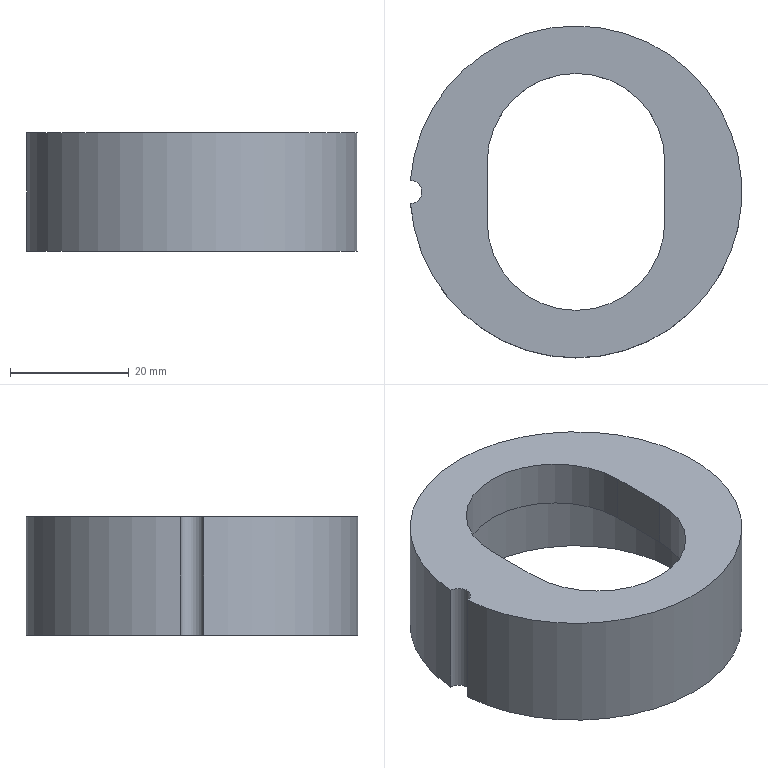Part | NX | features solid 2 | 1 solid | 10 faces | box 55.929 x 56 x 20 mm | volume 21139 mm3 | cylinder 5 | plane 5 | commonest cylinder face diameters 30 x2 4 x1 46 x1 56 x1
STEP:
#1=CARTESIAN_POINT('',(-627.931,-72.989,7.));
#2=VERTEX_POINT('',#1);
#3=CARTESIAN_POINT('',(-627.931,-72.989,27.));
#4=VERTEX_POINT('',#3);
#5=CARTESIAN_POINT('',(-627.931,-72.989,17.));
#6=DIRECTION('',(0.,0.,1.));
#7=VECTOR('',#6,1000.);
#8=LINE('',#5,#7);
#9=EDGE_CURVE('',#2,#4,#8,.T.);
#10=ORIENTED_EDGE('',*,*,#9,.F.);
#11=CARTESIAN_POINT('',(-627.931,-68.991,7.));
#12=VERTEX_POINT('',#11);
#13=CARTESIAN_POINT('',(-600.003,-70.99,7.));
#14=DIRECTION('',(0.,0.,1.));
#15=DIRECTION('',(-1.,0.,0.));
#16=AXIS2_PLACEMENT_3D('',#13,#14,#15);
#17=CIRCLE('',#16,28.);
#18=EDGE_CURVE('',#2,#12,#17,.T.);
#19=ORIENTED_EDGE('',*,*,#18,.T.);
#20=CARTESIAN_POINT('',(-627.931,-68.991,27.));
#21=VERTEX_POINT('',#20);
#22=CARTESIAN_POINT('',(-627.931,-68.991,17.));
#23=DIRECTION('',(0.,0.,1.));
#24=VECTOR('',#23,1000.);
#25=LINE('',#22,#24);
#26=EDGE_CURVE('',#21,#12,#25,.F.);
#27=ORIENTED_EDGE('',*,*,#26,.F.);
#28=CARTESIAN_POINT('',(-600.003,-70.99,27.));
#29=DIRECTION('',(0.,0.,1.));
#30=DIRECTION('',(-1.,0.,0.));
#31=AXIS2_PLACEMENT_3D('',#28,#29,#30);
#32=CIRCLE('',#31,28.);
#33=EDGE_CURVE('',#4,#21,#32,.T.);
#34=ORIENTED_EDGE('',*,*,#33,.F.);
#35=EDGE_LOOP('',(#10,#19,#27,#34));
#36=FACE_BOUND('',#35,.T.);
#37=CARTESIAN_POINT('',(-600.003,-70.99,7.));
#38=DIRECTION('',(0.,0.,1.));
#39=DIRECTION('',(-1.,0.,0.));
#40=AXIS2_PLACEMENT_3D('',#37,#38,#39);
#41=CYLINDRICAL_SURFACE('',#40,28.);
#42=ADVANCED_FACE('',(#36),#41,.T.);
#43=CARTESIAN_POINT('',(-623.003,-70.99,7.));
#44=VERTEX_POINT('',#43);
#45=CARTESIAN_POINT('',(-600.003,-70.99,7.));
#46=DIRECTION('',(0.,0.,1.));
#47=DIRECTION('',(-1.,0.,0.));
#48=AXIS2_PLACEMENT_3D('',#45,#46,#47);
#49=CIRCLE('',#48,23.);
#50=EDGE_CURVE('',#44,#44,#49,.T.);
#51=ORIENTED_EDGE('',*,*,#50,.T.);
#52=EDGE_LOOP('',(#51));
#53=FACE_BOUND('',#52,.T.);
#54=ORIENTED_EDGE('',*,*,#18,.F.);
#55=CARTESIAN_POINT('',(-628.003,-70.99,7.));
#56=DIRECTION('',(0.,0.,1.));
#57=DIRECTION('',(-1.,0.,0.));
#58=AXIS2_PLACEMENT_3D('',#55,#56,#57);
#59=CIRCLE('',#58,2.);
#60=EDGE_CURVE('',#2,#12,#59,.T.);
#61=ORIENTED_EDGE('',*,*,#60,.T.);
#62=EDGE_LOOP('',(#54,#61));
#63=FACE_BOUND('',#62,.T.);
#64=CARTESIAN_POINT('',(-600.003,-70.99,7.));
#65=DIRECTION('',(0.,0.,1.));
#66=DIRECTION('',(-1.,0.,0.));
#67=AXIS2_PLACEMENT_3D('',#64,#65,#66);
#68=PLANE('',#67);
#69=ADVANCED_FACE('',(#53,#63),#68,.F.);
#70=CARTESIAN_POINT('',(-585.003,-75.99,27.));
#71=VERTEX_POINT('',#70);
#72=CARTESIAN_POINT('',(-585.003,-65.99,27.));
#73=VERTEX_POINT('',#72);
#74=CARTESIAN_POINT('',(-585.003,-75.99,27.));
#75=DIRECTION('',(0.,1.,0.));
#76=VECTOR('',#75,1000.);
#77=LINE('',#74,#76);
#78=EDGE_CURVE('',#71,#73,#77,.T.);
#79=ORIENTED_EDGE('',*,*,#78,.F.);
#80=CARTESIAN_POINT('',(-615.003,-75.99,27.));
#81=VERTEX_POINT('',#80);
#82=CARTESIAN_POINT('',(-600.003,-75.99,27.));
#83=DIRECTION('',(0.,0.,1.));
#84=DIRECTION('',(-1.,0.,0.));
#85=AXIS2_PLACEMENT_3D('',#82,#83,#84);
#86=CIRCLE('',#85,15.);
#87=EDGE_CURVE('',#81,#71,#86,.T.);
#88=ORIENTED_EDGE('',*,*,#87,.F.);
#89=CARTESIAN_POINT('',(-615.003,-65.99,27.));
#90=VERTEX_POINT('',#89);
#91=CARTESIAN_POINT('',(-615.003,-75.99,27.));
#92=DIRECTION('',(0.,1.,0.));
#93=VECTOR('',#92,1000.);
#94=LINE('',#91,#93);
#95=EDGE_CURVE('',#81,#90,#94,.T.);
#96=ORIENTED_EDGE('',*,*,#95,.T.);
#97=CARTESIAN_POINT('',(-600.003,-65.99,27.));
#98=DIRECTION('',(0.,0.,1.));
#99=DIRECTION('',(-1.,0.,0.));
#100=AXIS2_PLACEMENT_3D('',#97,#98,#99);
#101=CIRCLE('',#100,15.);
#102=EDGE_CURVE('',#73,#90,#101,.T.);
#103=ORIENTED_EDGE('',*,*,#102,.F.);
#104=EDGE_LOOP('',(#79,#88,#96,#103));
#105=FACE_BOUND('',#104,.T.);
#106=CARTESIAN_POINT('',(-628.003,-70.99,27.));
#107=DIRECTION('',(0.,0.,1.));
#108=DIRECTION('',(-1.,0.,0.));
#109=AXIS2_PLACEMENT_3D('',#106,#107,#108);
#110=CIRCLE('',#109,2.);
#111=EDGE_CURVE('',#4,#21,#110,.T.);
#112=ORIENTED_EDGE('',*,*,#111,.F.);
#113=ORIENTED_EDGE('',*,*,#33,.T.);
#114=EDGE_LOOP('',(#112,#113));
#115=FACE_BOUND('',#114,.T.);
#116=CARTESIAN_POINT('',(-600.003,-70.99,27.));
#117=DIRECTION('',(0.,0.,1.));
#118=DIRECTION('',(-1.,0.,0.));
#119=AXIS2_PLACEMENT_3D('',#116,#117,#118);
#120=PLANE('',#119);
#121=ADVANCED_FACE('',(#105,#115),#120,.T.);
#122=ORIENTED_EDGE('',*,*,#50,.F.);
#123=EDGE_LOOP('',(#122));
#124=FACE_BOUND('',#123,.T.);
#125=CARTESIAN_POINT('',(-623.003,-70.99,19.));
#126=VERTEX_POINT('',#125);
#127=CARTESIAN_POINT('',(-600.003,-70.99,19.));
#128=DIRECTION('',(0.,0.,1.));
#129=DIRECTION('',(-1.,0.,0.));
#130=AXIS2_PLACEMENT_3D('',#127,#128,#129);
#131=CIRCLE('',#130,23.);
#132=EDGE_CURVE('',#126,#126,#131,.T.);
#133=ORIENTED_EDGE('',*,*,#132,.T.);
#134=EDGE_LOOP('',(#133));
#135=FACE_BOUND('',#134,.T.);
#136=CARTESIAN_POINT('',(-600.003,-70.99,7.));
#137=DIRECTION('',(0.,0.,1.));
#138=DIRECTION('',(-1.,0.,0.));
#139=AXIS2_PLACEMENT_3D('',#136,#137,#138);
#140=CYLINDRICAL_SURFACE('',#139,23.);
#141=ADVANCED_FACE('',(#124,#135),#140,.F.);
#142=CARTESIAN_POINT('',(-615.003,-75.99,19.));
#143=VERTEX_POINT('',#142);
#144=CARTESIAN_POINT('',(-585.003,-75.99,19.));
#145=VERTEX_POINT('',#144);
#146=CARTESIAN_POINT('',(-600.003,-75.99,19.));
#147=DIRECTION('',(0.,0.,1.));
#148=DIRECTION('',(-1.,0.,0.));
#149=AXIS2_PLACEMENT_3D('',#146,#147,#148);
#150=CIRCLE('',#149,15.);
#151=EDGE_CURVE('',#143,#145,#150,.T.);
#152=ORIENTED_EDGE('',*,*,#151,.T.);
#153=CARTESIAN_POINT('',(-585.003,-65.99,19.));
#154=VERTEX_POINT('',#153);
#155=CARTESIAN_POINT('',(-585.003,-70.99,19.));
#156=DIRECTION('',(0.,1.,0.));
#157=VECTOR('',#156,1000.);
#158=LINE('',#155,#157);
#159=EDGE_CURVE('',#145,#154,#158,.T.);
#160=ORIENTED_EDGE('',*,*,#159,.T.);
#161=CARTESIAN_POINT('',(-615.003,-65.99,19.));
#162=VERTEX_POINT('',#161);
#163=CARTESIAN_POINT('',(-600.003,-65.99,19.));
#164=DIRECTION('',(0.,0.,1.));
#165=DIRECTION('',(-1.,0.,0.));
#166=AXIS2_PLACEMENT_3D('',#163,#164,#165);
#167=CIRCLE('',#166,15.);
#168=EDGE_CURVE('',#154,#162,#167,.T.);
#169=ORIENTED_EDGE('',*,*,#168,.T.);
#170=CARTESIAN_POINT('',(-615.003,-70.99,19.));
#171=DIRECTION('',(0.,1.,0.));
#172=VECTOR('',#171,1000.);
#173=LINE('',#170,#172);
#174=EDGE_CURVE('',#143,#162,#173,.T.);
#175=ORIENTED_EDGE('',*,*,#174,.F.);
#176=EDGE_LOOP('',(#152,#160,#169,#175));
#177=FACE_BOUND('',#176,.T.);
#178=ORIENTED_EDGE('',*,*,#132,.F.);
#179=EDGE_LOOP('',(#178));
#180=FACE_BOUND('',#179,.T.);
#181=CARTESIAN_POINT('',(-600.003,-70.99,19.));
#182=DIRECTION('',(0.,0.,1.));
#183=DIRECTION('',(-1.,0.,0.));
#184=AXIS2_PLACEMENT_3D('',#181,#182,#183);
#185=PLANE('',#184);
#186=ADVANCED_FACE('',(#177,#180),#185,.F.);
#187=ORIENTED_EDGE('',*,*,#9,.T.);
#188=ORIENTED_EDGE('',*,*,#111,.T.);
#189=ORIENTED_EDGE('',*,*,#26,.T.);
#190=ORIENTED_EDGE('',*,*,#60,.F.);
#191=EDGE_LOOP('',(#187,#188,#189,#190));
#192=FACE_BOUND('',#191,.T.);
#193=CARTESIAN_POINT('',(-628.003,-70.99,7.));
#194=DIRECTION('',(0.,0.,1.));
#195=DIRECTION('',(-1.,0.,0.));
#196=AXIS2_PLACEMENT_3D('',#193,#194,#195);
#197=CYLINDRICAL_SURFACE('',#196,2.);
#198=ADVANCED_FACE('',(#192),#197,.F.);
#199=CARTESIAN_POINT('',(-585.003,-75.99,7.));
#200=DIRECTION('',(0.,0.,1.));
#201=VECTOR('',#200,1000.);
#202=LINE('',#199,#201);
#203=EDGE_CURVE('',#145,#71,#202,.T.);
#204=ORIENTED_EDGE('',*,*,#203,.T.);
#205=ORIENTED_EDGE('',*,*,#78,.T.);
#206=CARTESIAN_POINT('',(-585.003,-65.99,7.));
#207=DIRECTION('',(0.,0.,1.));
#208=VECTOR('',#207,1000.);
#209=LINE('',#206,#208);
#210=EDGE_CURVE('',#154,#73,#209,.T.);
#211=ORIENTED_EDGE('',*,*,#210,.F.);
#212=ORIENTED_EDGE('',*,*,#159,.F.);
#213=EDGE_LOOP('',(#204,#205,#211,#212));
#214=FACE_BOUND('',#213,.T.);
#215=CARTESIAN_POINT('',(-585.003,-75.99,7.));
#216=DIRECTION('',(1.,0.,0.));
#217=DIRECTION('',(0.,0.,1.));
#218=AXIS2_PLACEMENT_3D('',#215,#216,#217);
#219=PLANE('',#218);
#220=ADVANCED_FACE('',(#214),#219,.F.);
#221=ORIENTED_EDGE('',*,*,#210,.T.);
#222=ORIENTED_EDGE('',*,*,#102,.T.);
#223=CARTESIAN_POINT('',(-615.003,-65.99,7.));
#224=DIRECTION('',(0.,0.,1.));
#225=VECTOR('',#224,1000.);
#226=LINE('',#223,#225);
#227=EDGE_CURVE('',#162,#90,#226,.T.);
#228=ORIENTED_EDGE('',*,*,#227,.F.);
#229=ORIENTED_EDGE('',*,*,#168,.F.);
#230=EDGE_LOOP('',(#221,#222,#228,#229));
#231=FACE_BOUND('',#230,.T.);
#232=CARTESIAN_POINT('',(-600.003,-65.99,7.));
#233=DIRECTION('',(0.,0.,1.));
#234=DIRECTION('',(-1.,0.,0.));
#235=AXIS2_PLACEMENT_3D('',#232,#233,#234);
#236=CYLINDRICAL_SURFACE('',#235,15.);
#237=ADVANCED_FACE('',(#231),#236,.F.);
#238=ORIENTED_EDGE('',*,*,#174,.T.);
#239=ORIENTED_EDGE('',*,*,#227,.T.);
#240=ORIENTED_EDGE('',*,*,#95,.F.);
#241=CARTESIAN_POINT('',(-615.003,-75.99,7.));
#242=DIRECTION('',(0.,0.,1.));
#243=VECTOR('',#242,1000.);
#244=LINE('',#241,#243);
#245=EDGE_CURVE('',#143,#81,#244,.T.);
#246=ORIENTED_EDGE('',*,*,#245,.F.);
#247=EDGE_LOOP('',(#238,#239,#240,#246));
#248=FACE_BOUND('',#247,.T.);
#249=CARTESIAN_POINT('',(-615.003,-75.99,7.));
#250=DIRECTION('',(1.,0.,0.));
#251=DIRECTION('',(0.,0.,1.));
#252=AXIS2_PLACEMENT_3D('',#249,#250,#251);
#253=PLANE('',#252);
#254=ADVANCED_FACE('',(#248),#253,.T.);
#255=ORIENTED_EDGE('',*,*,#245,.T.);
#256=ORIENTED_EDGE('',*,*,#87,.T.);
#257=ORIENTED_EDGE('',*,*,#203,.F.);
#258=ORIENTED_EDGE('',*,*,#151,.F.);
#259=EDGE_LOOP('',(#255,#256,#257,#258));
#260=FACE_BOUND('',#259,.T.);
#261=CARTESIAN_POINT('',(-600.003,-75.99,7.));
#262=DIRECTION('',(0.,0.,1.));
#263=DIRECTION('',(-1.,0.,0.));
#264=AXIS2_PLACEMENT_3D('',#261,#262,#263);
#265=CYLINDRICAL_SURFACE('',#264,15.);
#266=ADVANCED_FACE('',(#260),#265,.F.);
#267=CLOSED_SHELL('',(#42,#69,#121,#141,#186,#198,#220,#237,#254,#266));
#268=MANIFOLD_SOLID_BREP('',#267);
#269=(LENGTH_UNIT()NAMED_UNIT(*)SI_UNIT(.MILLI.,.METRE.));
#270=UNCERTAINTY_MEASURE_WITH_UNIT(LENGTH_MEASURE(0.00001),#269,'','');
#271=(NAMED_UNIT(*)PLANE_ANGLE_UNIT()SI_UNIT($,.RADIAN.));
#272=(NAMED_UNIT(*)SI_UNIT($,.STERADIAN.)SOLID_ANGLE_UNIT());
#273=(GEOMETRIC_REPRESENTATION_CONTEXT(3)GLOBAL_UNCERTAINTY_ASSIGNED_CONTEXT((#270))GLOBAL_UNIT_ASSIGNED_CONTEXT((#269,#271,#272))REPRESENTATION_CONTEXT('',''));
#274=ADVANCED_BREP_SHAPE_REPRESENTATION('',(#268),#273);